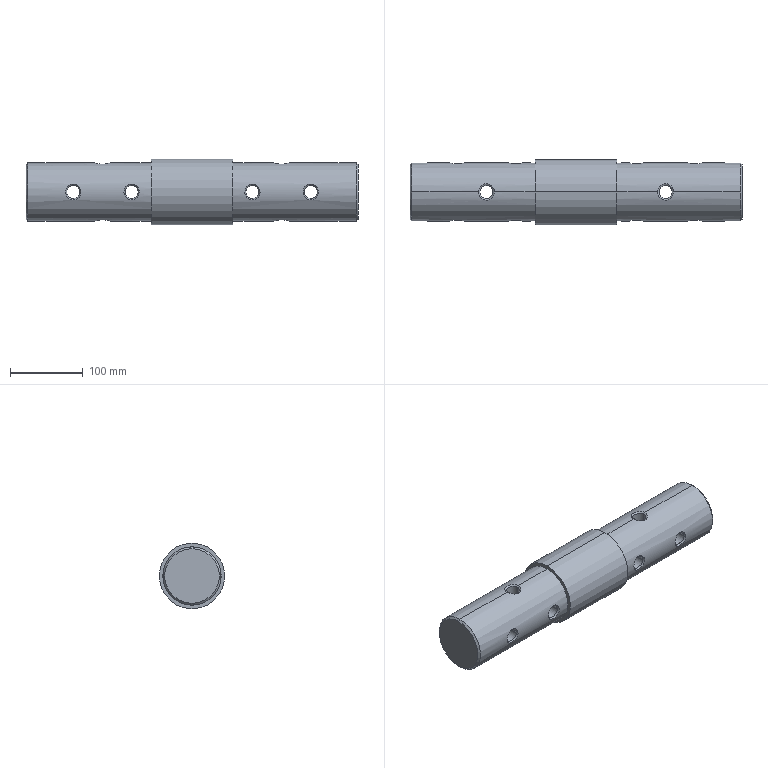Part | STEP file | Input 129 | 1 solid | 50 faces | box 456 x 90 x 90 mm | volume 2317318 mm3 | spline 24 | cylinder 18 | cone 4 | plane 4 | commonest cylinder face diameters 18 x12 80 x4 90 x2